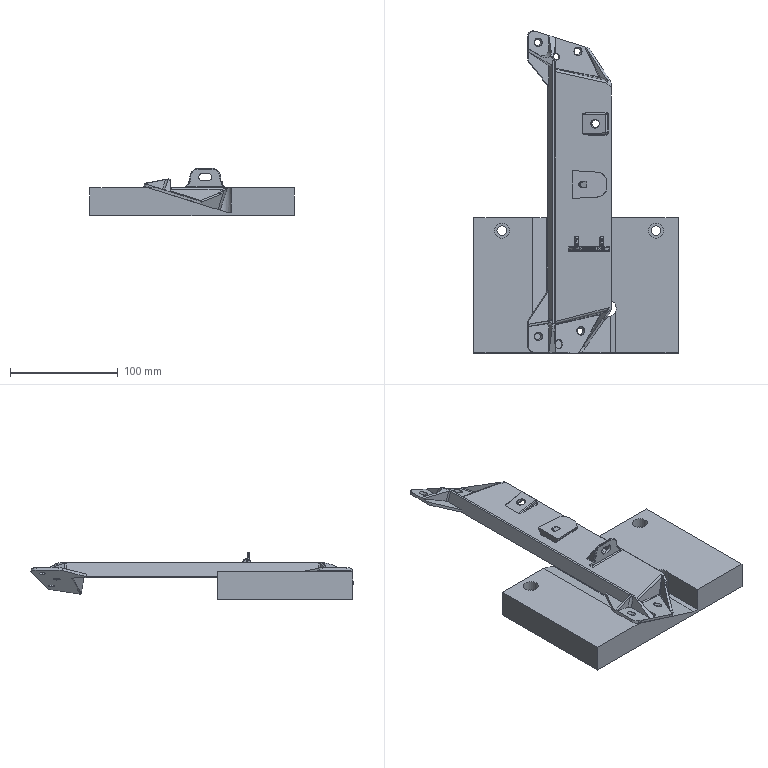CAM job | NX | 3-axis milling | part box 190 x 299.709 x 43.804 mm
Tools:
number,name,description,diameter,corner_radius,flute_length,length,flutes
1,D6-粗刀,D6-粗刀-L,6.0,0.0,40.0,40.0,2
3,D4,Milling Tool-5 Parameters,4.0,0.0,100.0,100.0,2
4,R3,Milling Tool-Ball Mill,6.0,3.0,50.0,75.0,2
Operations:
program,operation,operation_type,tool,method,geometry_group,spindle_rpm,surface_speed,feed_per_tooth,feed_cut,feed_plunge,cut_length_mm,path_length_mm,cut_time_min,machine_time_min
1,G-型腔铣-粗,CavityMilling,D6-粗刀,METHOD,MCS_MAIN,5300.0,99.0,0.217,2300.0,100.0,7937.379,14952.671,3.451,4.153
1,G-型腔铣-粗_COPY,CavityMilling,D6-粗刀,METHOD,MCS_MAIN,5300.0,99.0,0.217,2300.0,100.0,14881.039,23458.12,6.47,7.328
2,L等高精加工_COPY_COPY,ZLevelMilling,D6-粗刀,METHOD,MCS_MAIN_COPY,6000.0,113.0,0.1111,2000.0,100.0,2060.046,2112.38,1.03,1.035
3,VARIABLE_AXIS_GUIDING_CURVES,SurfaceContour,R3,METHOD,A,6800.0,128.177,0.1838,2500.0,100.0,653.819,898.644,0.2615,0.286
01,PLANAR_MILL_4_COPY_COPY_2_COPY_COPY_1_COPY,PlanarMilling,D4,METHOD,MCS_MAIN_COPY,5800.0,72.885,0.2155,2500.0,100.0,628.674,841.95,0.2515,0.2728
01,PLANAR_MILL_4_COPY_COPY_2_COPY_COPY_1_COPY_COPY,PlanarMilling,D4,METHOD,MCS_MAIN_COPY,5800.0,72.885,0.069,800.0,100.0,23.573,239.34,0.0295,0.051